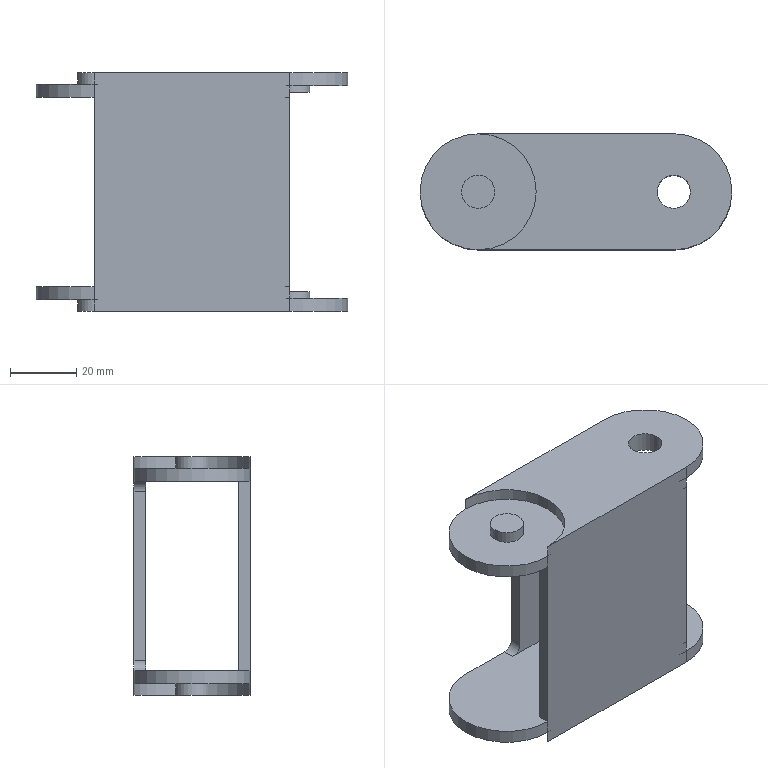Part | STEP file | 1 solid | 40 faces | box 94 x 35 x 72 mm | volume 47784 mm3 | plane 22 | cylinder 18 | commonest cylinder face diameters 35 x8 6 x4 10 x4 12 x2